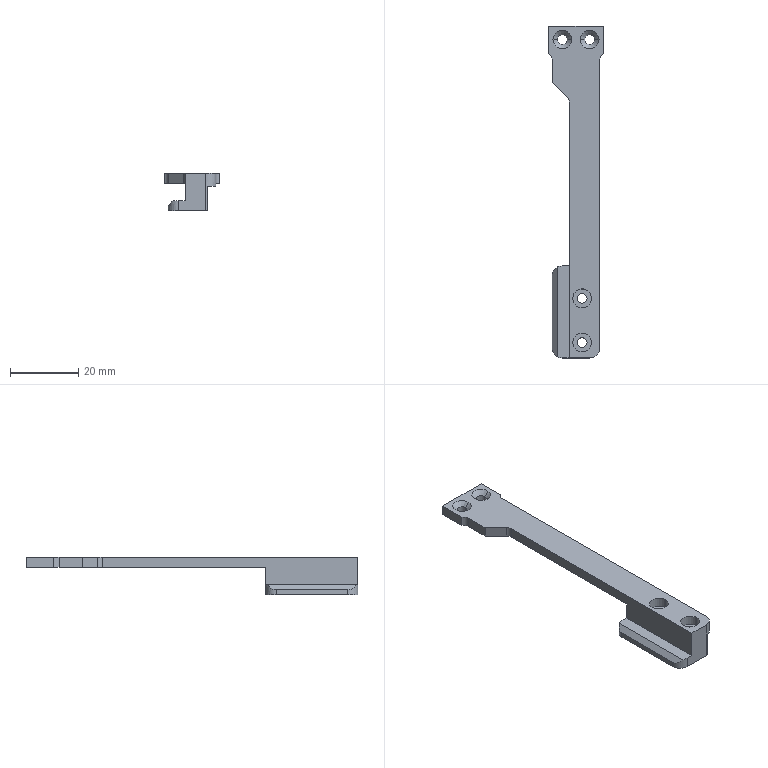Part | 1 solid | 42 faces | box 16 x 97.4 x 11 mm | volume 4478 mm3 | plane 19 | cylinder 19 | cone 4 | commonest cylinder face diameters 2.9 x8 5.5 x4 6 x4 4 x3
STEP:
#1=CARTESIAN_POINT('',(14.,3.,7.2));
#2=VERTEX_POINT('',#1);
#3=CARTESIAN_POINT('',(11.5,0.04196,7.2));
#4=VERTEX_POINT('',#3);
#5=CARTESIAN_POINT('',(11.,3.,7.2));
#6=DIRECTION('',(0.,0.,-1.));
#7=DIRECTION('',(0.,-1.,0.));
#8=AXIS2_PLACEMENT_3D('',#5,#6,#7);
#9=CIRCLE('',#8,3.);
#10=EDGE_CURVE('',#2,#4,#9,.T.);
#11=ORIENTED_EDGE('',*,*,#10,.T.);
#12=CARTESIAN_POINT('',(11.5,26.958,7.2));
#13=VERTEX_POINT('',#12);
#14=CARTESIAN_POINT('',(11.5,29.,7.2));
#15=DIRECTION('',(0.,-1.,0.));
#16=VECTOR('',#15,1000.);
#17=LINE('',#14,#16);
#18=EDGE_CURVE('',#13,#4,#17,.T.);
#19=ORIENTED_EDGE('',*,*,#18,.F.);
#20=CARTESIAN_POINT('',(14.,24.,7.2));
#21=VERTEX_POINT('',#20);
#22=CARTESIAN_POINT('',(11.,24.,7.2));
#23=DIRECTION('',(0.,0.,-1.));
#24=DIRECTION('',(0.,-1.,0.));
#25=AXIS2_PLACEMENT_3D('',#22,#23,#24);
#26=CIRCLE('',#25,3.);
#27=EDGE_CURVE('',#13,#21,#26,.T.);
#28=ORIENTED_EDGE('',*,*,#27,.T.);
#29=CARTESIAN_POINT('',(14.,29.,7.2));
#30=DIRECTION('',(0.,-1.,0.));
#31=VECTOR('',#30,1000.);
#32=LINE('',#29,#31);
#33=EDGE_CURVE('',#21,#2,#32,.T.);
#34=ORIENTED_EDGE('',*,*,#33,.T.);
#35=EDGE_LOOP('',(#11,#19,#28,#34));
#36=FACE_BOUND('',#35,.T.);
#37=CARTESIAN_POINT('',(14.,29.,7.2));
#38=DIRECTION('',(0.,0.,1.));
#39=DIRECTION('',(0.,-1.,0.));
#40=AXIS2_PLACEMENT_3D('',#37,#38,#39);
#41=PLANE('',#40);
#42=ADVANCED_FACE('',(#36),#41,.F.);
#43=CARTESIAN_POINT('',(11.5,0.04196,0.));
#44=VERTEX_POINT('',#43);
#45=CARTESIAN_POINT('',(11.5,0.04196,0.));
#46=DIRECTION('',(0.,0.,-1.));
#47=VECTOR('',#46,1000.);
#48=LINE('',#45,#47);
#49=EDGE_CURVE('',#4,#44,#48,.T.);
#50=ORIENTED_EDGE('',*,*,#49,.T.);
#51=CARTESIAN_POINT('',(11.5,26.958,0.));
#52=VERTEX_POINT('',#51);
#53=CARTESIAN_POINT('',(11.5,29.,0.));
#54=DIRECTION('',(0.,-1.,0.));
#55=VECTOR('',#54,1000.);
#56=LINE('',#53,#55);
#57=EDGE_CURVE('',#52,#44,#56,.T.);
#58=ORIENTED_EDGE('',*,*,#57,.F.);
#59=CARTESIAN_POINT('',(11.5,26.958,0.));
#60=DIRECTION('',(0.,0.,1.));
#61=VECTOR('',#60,1000.);
#62=LINE('',#59,#61);
#63=EDGE_CURVE('',#52,#13,#62,.T.);
#64=ORIENTED_EDGE('',*,*,#63,.T.);
#65=ORIENTED_EDGE('',*,*,#18,.T.);
#66=EDGE_LOOP('',(#50,#58,#64,#65));
#67=FACE_BOUND('',#66,.T.);
#68=CARTESIAN_POINT('',(11.5,29.,0.));
#69=DIRECTION('',(-1.,0.,0.));
#70=DIRECTION('',(0.,-1.,0.));
#71=AXIS2_PLACEMENT_3D('',#68,#69,#70);
#72=PLANE('',#71);
#73=ADVANCED_FACE('',(#67),#72,.F.);
#74=CARTESIAN_POINT('',(-1.,89.4,11.));
#75=VERTEX_POINT('',#74);
#76=CARTESIAN_POINT('',(0.,87.668,11.));
#77=VERTEX_POINT('',#76);
#78=CARTESIAN_POINT('',(-2.,87.668,11.));
#79=DIRECTION('',(0.,0.,-1.));
#80=DIRECTION('',(1.,0.,0.));
#81=AXIS2_PLACEMENT_3D('',#78,#79,#80);
#82=CIRCLE('',#81,2.);
#83=EDGE_CURVE('',#75,#77,#82,.T.);
#84=ORIENTED_EDGE('',*,*,#83,.F.);
#85=CARTESIAN_POINT('',(-1.,89.4,8.));
#86=VERTEX_POINT('',#85);
#87=CARTESIAN_POINT('',(-1.,89.4,-9.889));
#88=DIRECTION('',(0.,0.,1.));
#89=VECTOR('',#88,1000.);
#90=LINE('',#87,#89);
#91=EDGE_CURVE('',#86,#75,#90,.T.);
#92=ORIENTED_EDGE('',*,*,#91,.F.);
#93=CARTESIAN_POINT('',(0.,87.668,8.));
#94=VERTEX_POINT('',#93);
#95=CARTESIAN_POINT('',(-2.,87.668,8.));
#96=DIRECTION('',(0.,0.,1.));
#97=DIRECTION('',(1.,0.,0.));
#98=AXIS2_PLACEMENT_3D('',#95,#96,#97);
#99=CIRCLE('',#98,2.);
#100=EDGE_CURVE('',#94,#86,#99,.T.);
#101=ORIENTED_EDGE('',*,*,#100,.F.);
#102=CARTESIAN_POINT('',(0.,87.668,3.));
#103=DIRECTION('',(0.,0.,-1.));
#104=VECTOR('',#103,1000.);
#105=LINE('',#102,#104);
#106=EDGE_CURVE('',#77,#94,#105,.T.);
#107=ORIENTED_EDGE('',*,*,#106,.F.);
#108=EDGE_LOOP('',(#84,#92,#101,#107));
#109=FACE_BOUND('',#108,.T.);
#110=CARTESIAN_POINT('',(-2.,87.668,-9.889));
#111=DIRECTION('',(0.,0.,-1.));
#112=DIRECTION('',(-1.,0.,0.));
#113=AXIS2_PLACEMENT_3D('',#110,#111,#112);
#114=CYLINDRICAL_SURFACE('',#113,2.);
#115=ADVANCED_FACE('',(#109),#114,.F.);
#116=CARTESIAN_POINT('',(15.,89.4,8.));
#117=VERTEX_POINT('',#116);
#118=CARTESIAN_POINT('',(14.,87.668,8.));
#119=VERTEX_POINT('',#118);
#120=CARTESIAN_POINT('',(16.,87.668,8.));
#121=DIRECTION('',(0.,0.,1.));
#122=DIRECTION('',(1.,0.,0.));
#123=AXIS2_PLACEMENT_3D('',#120,#121,#122);
#124=CIRCLE('',#123,2.);
#125=EDGE_CURVE('',#117,#119,#124,.T.);
#126=ORIENTED_EDGE('',*,*,#125,.F.);
#127=CARTESIAN_POINT('',(15.,89.4,11.));
#128=VERTEX_POINT('',#127);
#129=CARTESIAN_POINT('',(15.,89.4,-9.889));
#130=DIRECTION('',(0.,0.,1.));
#131=VECTOR('',#130,1000.);
#132=LINE('',#129,#131);
#133=EDGE_CURVE('',#117,#128,#132,.T.);
#134=ORIENTED_EDGE('',*,*,#133,.T.);
#135=CARTESIAN_POINT('',(14.,87.668,11.));
#136=VERTEX_POINT('',#135);
#137=CARTESIAN_POINT('',(16.,87.668,11.));
#138=DIRECTION('',(0.,0.,-1.));
#139=DIRECTION('',(1.,0.,0.));
#140=AXIS2_PLACEMENT_3D('',#137,#138,#139);
#141=CIRCLE('',#140,2.);
#142=EDGE_CURVE('',#136,#128,#141,.T.);
#143=ORIENTED_EDGE('',*,*,#142,.F.);
#144=CARTESIAN_POINT('',(14.,87.668,0.));
#145=DIRECTION('',(0.,0.,1.));
#146=VECTOR('',#145,1000.);
#147=LINE('',#144,#146);
#148=EDGE_CURVE('',#119,#136,#147,.T.);
#149=ORIENTED_EDGE('',*,*,#148,.F.);
#150=EDGE_LOOP('',(#126,#134,#143,#149));
#151=FACE_BOUND('',#150,.T.);
#152=CARTESIAN_POINT('',(16.,87.668,-9.889));
#153=DIRECTION('',(0.,0.,1.));
#154=DIRECTION('',(1.,0.,0.));
#155=AXIS2_PLACEMENT_3D('',#152,#153,#154);
#156=CYLINDRICAL_SURFACE('',#155,2.);
#157=ADVANCED_FACE('',(#151),#156,.F.);
#158=CARTESIAN_POINT('',(1.55,93.4,9.7));
#159=VERTEX_POINT('',#158);
#160=CARTESIAN_POINT('',(0.25,93.4,11.));
#161=VERTEX_POINT('',#160);
#162=CARTESIAN_POINT('',(0.25,93.4,11.));
#163=DIRECTION('',(-0.7071,0.,0.7071));
#164=VECTOR('',#163,1000.);
#165=LINE('',#162,#164);
#166=EDGE_CURVE('',#159,#161,#165,.T.);
#167=ORIENTED_EDGE('',*,*,#166,.F.);
#168=CARTESIAN_POINT('',(4.45,93.4,9.7));
#169=VERTEX_POINT('',#168);
#170=CARTESIAN_POINT('',(3.,93.4,9.7));
#171=DIRECTION('',(0.,0.,1.));
#172=DIRECTION('',(1.,0.,0.));
#173=AXIS2_PLACEMENT_3D('',#170,#171,#172);
#174=CIRCLE('',#173,1.45);
#175=EDGE_CURVE('',#169,#159,#174,.T.);
#176=ORIENTED_EDGE('',*,*,#175,.F.);
#177=CARTESIAN_POINT('',(5.75,93.4,11.));
#178=VERTEX_POINT('',#177);
#179=CARTESIAN_POINT('',(5.75,93.4,11.));
#180=DIRECTION('',(0.7071,0.,0.7071));
#181=VECTOR('',#180,1000.);
#182=LINE('',#179,#181);
#183=EDGE_CURVE('',#169,#178,#182,.T.);
#184=ORIENTED_EDGE('',*,*,#183,.T.);
#185=CARTESIAN_POINT('',(3.,93.4,11.));
#186=DIRECTION('',(0.,0.,1.));
#187=DIRECTION('',(1.,0.,0.));
#188=AXIS2_PLACEMENT_3D('',#185,#186,#187);
#189=CIRCLE('',#188,2.75);
#190=EDGE_CURVE('',#178,#161,#189,.T.);
#191=ORIENTED_EDGE('',*,*,#190,.T.);
#192=EDGE_LOOP('',(#167,#176,#184,#191));
#193=FACE_BOUND('',#192,.T.);
#194=CARTESIAN_POINT('',(3.,93.4,11.));
#195=DIRECTION('',(0.,0.,1.));
#196=DIRECTION('',(1.,0.,0.));
#197=AXIS2_PLACEMENT_3D('',#194,#195,#196);
#198=CONICAL_SURFACE('',#197,2.75,0.7854);
#199=ADVANCED_FACE('',(#193),#198,.F.);
#200=CARTESIAN_POINT('',(1.55,93.4,8.));
#201=VERTEX_POINT('',#200);
#202=CARTESIAN_POINT('',(1.55,93.4,11.));
#203=DIRECTION('',(0.,0.,1.));
#204=VECTOR('',#203,1000.);
#205=LINE('',#202,#204);
#206=EDGE_CURVE('',#201,#159,#205,.T.);
#207=ORIENTED_EDGE('',*,*,#206,.F.);
#208=CARTESIAN_POINT('',(4.45,93.4,8.));
#209=VERTEX_POINT('',#208);
#210=CARTESIAN_POINT('',(3.,93.4,8.));
#211=DIRECTION('',(0.,0.,1.));
#212=DIRECTION('',(1.,0.,0.));
#213=AXIS2_PLACEMENT_3D('',#210,#211,#212);
#214=CIRCLE('',#213,1.45);
#215=EDGE_CURVE('',#209,#201,#214,.T.);
#216=ORIENTED_EDGE('',*,*,#215,.F.);
#217=CARTESIAN_POINT('',(4.45,93.4,11.));
#218=DIRECTION('',(0.,0.,1.));
#219=VECTOR('',#218,1000.);
#220=LINE('',#217,#219);
#221=EDGE_CURVE('',#209,#169,#220,.T.);
#222=ORIENTED_EDGE('',*,*,#221,.T.);
#223=ORIENTED_EDGE('',*,*,#175,.T.);
#224=EDGE_LOOP('',(#207,#216,#222,#223));
#225=FACE_BOUND('',#224,.T.);
#226=CARTESIAN_POINT('',(3.,93.4,11.));
#227=DIRECTION('',(0.,0.,1.));
#228=DIRECTION('',(1.,0.,0.));
#229=AXIS2_PLACEMENT_3D('',#226,#227,#228);
#230=CYLINDRICAL_SURFACE('',#229,1.45);
#231=ADVANCED_FACE('',(#225),#230,.F.);
#232=CARTESIAN_POINT('',(9.55,93.4,9.7));
#233=VERTEX_POINT('',#232);
#234=CARTESIAN_POINT('',(8.25,93.4,11.));
#235=VERTEX_POINT('',#234);
#236=CARTESIAN_POINT('',(8.25,93.4,11.));
#237=DIRECTION('',(-0.7071,0.,0.7071));
#238=VECTOR('',#237,1000.);
#239=LINE('',#236,#238);
#240=EDGE_CURVE('',#233,#235,#239,.T.);
#241=ORIENTED_EDGE('',*,*,#240,.F.);
#242=CARTESIAN_POINT('',(12.45,93.4,9.7));
#243=VERTEX_POINT('',#242);
#244=CARTESIAN_POINT('',(11.,93.4,9.7));
#245=DIRECTION('',(0.,0.,1.));
#246=DIRECTION('',(1.,0.,0.));
#247=AXIS2_PLACEMENT_3D('',#244,#245,#246);
#248=CIRCLE('',#247,1.45);
#249=EDGE_CURVE('',#243,#233,#248,.T.);
#250=ORIENTED_EDGE('',*,*,#249,.F.);
#251=CARTESIAN_POINT('',(13.75,93.4,11.));
#252=VERTEX_POINT('',#251);
#253=CARTESIAN_POINT('',(13.75,93.4,11.));
#254=DIRECTION('',(0.7071,0.,0.7071));
#255=VECTOR('',#254,1000.);
#256=LINE('',#253,#255);
#257=EDGE_CURVE('',#243,#252,#256,.T.);
#258=ORIENTED_EDGE('',*,*,#257,.T.);
#259=CARTESIAN_POINT('',(11.,93.4,11.));
#260=DIRECTION('',(0.,0.,1.));
#261=DIRECTION('',(1.,0.,0.));
#262=AXIS2_PLACEMENT_3D('',#259,#260,#261);
#263=CIRCLE('',#262,2.75);
#264=EDGE_CURVE('',#252,#235,#263,.T.);
#265=ORIENTED_EDGE('',*,*,#264,.T.);
#266=EDGE_LOOP('',(#241,#250,#258,#265));
#267=FACE_BOUND('',#266,.T.);
#268=CARTESIAN_POINT('',(11.,93.4,11.));
#269=DIRECTION('',(0.,0.,1.));
#270=DIRECTION('',(1.,0.,0.));
#271=AXIS2_PLACEMENT_3D('',#268,#269,#270);
#272=CONICAL_SURFACE('',#271,2.75,0.7854);
#273=ADVANCED_FACE('',(#267),#272,.F.);
#274=CARTESIAN_POINT('',(9.55,93.4,8.));
#275=VERTEX_POINT('',#274);
#276=CARTESIAN_POINT('',(9.55,93.4,11.));
#277=DIRECTION('',(0.,0.,1.));
#278=VECTOR('',#277,1000.);
#279=LINE('',#276,#278);
#280=EDGE_CURVE('',#275,#233,#279,.T.);
#281=ORIENTED_EDGE('',*,*,#280,.F.);
#282=CARTESIAN_POINT('',(12.45,93.4,8.));
#283=VERTEX_POINT('',#282);
#284=CARTESIAN_POINT('',(11.,93.4,8.));
#285=DIRECTION('',(0.,0.,1.));
#286=DIRECTION('',(1.,0.,0.));
#287=AXIS2_PLACEMENT_3D('',#284,#285,#286);
#288=CIRCLE('',#287,1.45);
#289=EDGE_CURVE('',#283,#275,#288,.T.);
#290=ORIENTED_EDGE('',*,*,#289,.F.);
#291=CARTESIAN_POINT('',(12.45,93.4,11.));
#292=DIRECTION('',(0.,0.,1.));
#293=VECTOR('',#292,1000.);
#294=LINE('',#291,#293);
#295=EDGE_CURVE('',#283,#243,#294,.T.);
#296=ORIENTED_EDGE('',*,*,#295,.T.);
#297=ORIENTED_EDGE('',*,*,#249,.T.);
#298=EDGE_LOOP('',(#281,#290,#296,#297));
#299=FACE_BOUND('',#298,.T.);
#300=CARTESIAN_POINT('',(11.,93.4,11.));
#301=DIRECTION('',(0.,0.,1.));
#302=DIRECTION('',(1.,0.,0.));
#303=AXIS2_PLACEMENT_3D('',#300,#301,#302);
#304=CYLINDRICAL_SURFACE('',#303,1.45);
#305=ADVANCED_FACE('',(#299),#304,.F.);
#306=CARTESIAN_POINT('',(-1.,97.4,8.));
#307=VERTEX_POINT('',#306);
#308=CARTESIAN_POINT('',(-1.,97.4,8.));
#309=DIRECTION('',(0.,1.,0.));
#310=VECTOR('',#309,1000.);
#311=LINE('',#308,#310);
#312=EDGE_CURVE('',#86,#307,#311,.T.);
#313=ORIENTED_EDGE('',*,*,#312,.F.);
#314=ORIENTED_EDGE('',*,*,#91,.T.);
#315=CARTESIAN_POINT('',(-1.,97.4,11.));
#316=VERTEX_POINT('',#315);
#317=CARTESIAN_POINT('',(-1.,97.4,11.));
#318=DIRECTION('',(0.,-1.,0.));
#319=VECTOR('',#318,1000.);
#320=LINE('',#317,#319);
#321=EDGE_CURVE('',#316,#75,#320,.T.);
#322=ORIENTED_EDGE('',*,*,#321,.F.);
#323=CARTESIAN_POINT('',(-1.,97.4,-9.889));
#324=DIRECTION('',(0.,0.,1.));
#325=VECTOR('',#324,1000.);
#326=LINE('',#323,#325);
#327=EDGE_CURVE('',#307,#316,#326,.T.);
#328=ORIENTED_EDGE('',*,*,#327,.F.);
#329=EDGE_LOOP('',(#313,#314,#322,#328));
#330=FACE_BOUND('',#329,.T.);
#331=CARTESIAN_POINT('',(-1.,97.4,-9.889));
#332=DIRECTION('',(-1.,0.,0.));
#333=DIRECTION('',(0.,-1.,0.));
#334=AXIS2_PLACEMENT_3D('',#331,#332,#333);
#335=PLANE('',#334);
#336=ADVANCED_FACE('',(#330),#335,.T.);
#337=CARTESIAN_POINT('',(15.,97.4,8.));
#338=VERTEX_POINT('',#337);
#339=CARTESIAN_POINT('',(15.,97.4,8.));
#340=DIRECTION('',(0.,-1.,0.));
#341=VECTOR('',#340,1000.);
#342=LINE('',#339,#341);
#343=EDGE_CURVE('',#338,#117,#342,.T.);
#344=ORIENTED_EDGE('',*,*,#343,.F.);
#345=CARTESIAN_POINT('',(15.,97.4,11.));
#346=VERTEX_POINT('',#345);
#347=CARTESIAN_POINT('',(15.,97.4,-9.889));
#348=DIRECTION('',(0.,0.,1.));
#349=VECTOR('',#348,1000.);
#350=LINE('',#347,#349);
#351=EDGE_CURVE('',#338,#346,#350,.T.);
#352=ORIENTED_EDGE('',*,*,#351,.T.);
#353=CARTESIAN_POINT('',(15.,97.4,11.));
#354=DIRECTION('',(0.,1.,0.));
#355=VECTOR('',#354,1000.);
#356=LINE('',#353,#355);
#357=EDGE_CURVE('',#128,#346,#356,.T.);
#358=ORIENTED_EDGE('',*,*,#357,.F.);
#359=ORIENTED_EDGE('',*,*,#133,.F.);
#360=EDGE_LOOP('',(#344,#352,#358,#359));
#361=FACE_BOUND('',#360,.T.);
#362=CARTESIAN_POINT('',(15.,97.4,-9.889));
#363=DIRECTION('',(1.,0.,0.));
#364=DIRECTION('',(0.,1.,0.));
#365=AXIS2_PLACEMENT_3D('',#362,#363,#364);
#366=PLANE('',#365);
#367=ADVANCED_FACE('',(#361),#366,.T.);
#368=CARTESIAN_POINT('',(5.,75.005,8.));
#369=VERTEX_POINT('',#368);
#370=CARTESIAN_POINT('',(4.414,76.419,8.));
#371=VERTEX_POINT('',#370);
#372=CARTESIAN_POINT('',(3.,75.005,8.));
#373=DIRECTION('',(0.,0.,1.));
#374=DIRECTION('',(1.,0.,0.));
#375=AXIS2_PLACEMENT_3D('',#372,#373,#374);
#376=CIRCLE('',#375,2.);
#377=EDGE_CURVE('',#369,#371,#376,.T.);
#378=ORIENTED_EDGE('',*,*,#377,.F.);
#379=CARTESIAN_POINT('',(5.,75.005,11.));
#380=VERTEX_POINT('',#379);
#381=CARTESIAN_POINT('',(5.,75.005,8.));
#382=DIRECTION('',(0.,0.,-1.));
#383=VECTOR('',#382,1000.);
#384=LINE('',#381,#383);
#385=EDGE_CURVE('',#380,#369,#384,.T.);
#386=ORIENTED_EDGE('',*,*,#385,.F.);
#387=CARTESIAN_POINT('',(4.414,76.419,11.));
#388=VERTEX_POINT('',#387);
#389=CARTESIAN_POINT('',(3.,75.005,11.));
#390=DIRECTION('',(0.,0.,-1.));
#391=DIRECTION('',(1.,0.,0.));
#392=AXIS2_PLACEMENT_3D('',#389,#390,#391);
#393=CIRCLE('',#392,2.);
#394=EDGE_CURVE('',#388,#380,#393,.T.);
#395=ORIENTED_EDGE('',*,*,#394,.F.);
#396=CARTESIAN_POINT('',(4.414,76.419,11.));
#397=DIRECTION('',(0.,0.,1.));
#398=VECTOR('',#397,1000.);
#399=LINE('',#396,#398);
#400=EDGE_CURVE('',#371,#388,#399,.T.);
#401=ORIENTED_EDGE('',*,*,#400,.F.);
#402=EDGE_LOOP('',(#378,#386,#395,#401));
#403=FACE_BOUND('',#402,.T.);
#404=CARTESIAN_POINT('',(3.,75.005,3.));
#405=DIRECTION('',(0.,0.,-1.));
#406=DIRECTION('',(-1.,0.,0.));
#407=AXIS2_PLACEMENT_3D('',#404,#405,#406);
#408=CYLINDRICAL_SURFACE('',#407,2.);
#409=ADVANCED_FACE('',(#403),#408,.F.);
#410=CARTESIAN_POINT('',(6.049,4.5,8.1));
#411=VERTEX_POINT('',#410);
#412=CARTESIAN_POINT('',(6.049,4.5,11.));
#413=VERTEX_POINT('',#412);
#414=CARTESIAN_POINT('',(6.049,4.5,11.));
#415=DIRECTION('',(0.,0.,1.));
#416=VECTOR('',#415,1000.);
#417=LINE('',#414,#416);
#418=EDGE_CURVE('',#411,#413,#417,.T.);
#419=ORIENTED_EDGE('',*,*,#418,.F.);
#420=CARTESIAN_POINT('',(11.549,4.5,8.1));
#421=VERTEX_POINT('',#420);
#422=CARTESIAN_POINT('',(8.799,4.5,8.1));
#423=DIRECTION('',(0.,0.,1.));
#424=DIRECTION('',(1.,0.,0.));
#425=AXIS2_PLACEMENT_3D('',#422,#423,#424);
#426=CIRCLE('',#425,2.75);
#427=EDGE_CURVE('',#421,#411,#426,.T.);
#428=ORIENTED_EDGE('',*,*,#427,.F.);
#429=CARTESIAN_POINT('',(11.549,4.5,11.));
#430=VERTEX_POINT('',#429);
#431=CARTESIAN_POINT('',(11.549,4.5,11.));
#432=DIRECTION('',(0.,0.,1.));
#433=VECTOR('',#432,1000.);
#434=LINE('',#431,#433);
#435=EDGE_CURVE('',#421,#430,#434,.T.);
#436=ORIENTED_EDGE('',*,*,#435,.T.);
#437=CARTESIAN_POINT('',(8.799,4.5,11.));
#438=DIRECTION('',(0.,0.,1.));
#439=DIRECTION('',(1.,0.,0.));
#440=AXIS2_PLACEMENT_3D('',#437,#438,#439);
#441=CIRCLE('',#440,2.75);
#442=EDGE_CURVE('',#430,#413,#441,.T.);
#443=ORIENTED_EDGE('',*,*,#442,.T.);
#444=EDGE_LOOP('',(#419,#428,#436,#443));
#445=FACE_BOUND('',#444,.T.);
#446=CARTESIAN_POINT('',(8.799,4.5,11.));
#447=DIRECTION('',(0.,0.,1.));
#448=DIRECTION('',(1.,0.,0.));
#449=AXIS2_PLACEMENT_3D('',#446,#447,#448);
#450=CYLINDRICAL_SURFACE('',#449,2.75);
#451=ADVANCED_FACE('',(#445),#450,.F.);
#452=ORIENTED_EDGE('',*,*,#427,.T.);
#453=CARTESIAN_POINT('',(8.799,4.5,8.1));
#454=DIRECTION('',(0.,0.,1.));
#455=DIRECTION('',(1.,0.,0.));
#456=AXIS2_PLACEMENT_3D('',#453,#454,#455);
#457=CIRCLE('',#456,2.75);
#458=EDGE_CURVE('',#411,#421,#457,.T.);
#459=ORIENTED_EDGE('',*,*,#458,.T.);
#460=EDGE_LOOP('',(#452,#459));
#461=FACE_BOUND('',#460,.T.);
#462=CARTESIAN_POINT('',(10.249,4.5,8.1));
#463=VERTEX_POINT('',#462);
#464=CARTESIAN_POINT('',(7.349,4.5,8.1));
#465=VERTEX_POINT('',#464);
#466=CARTESIAN_POINT('',(8.799,4.5,8.1));
#467=DIRECTION('',(0.,0.,1.));
#468=DIRECTION('',(1.,0.,0.));
#469=AXIS2_PLACEMENT_3D('',#466,#467,#468);
#470=CIRCLE('',#469,1.45);
#471=EDGE_CURVE('',#463,#465,#470,.T.);
#472=ORIENTED_EDGE('',*,*,#471,.F.);
#473=CARTESIAN_POINT('',(8.799,4.5,8.1));
#474=DIRECTION('',(0.,0.,1.));
#475=DIRECTION('',(1.,0.,0.));
#476=AXIS2_PLACEMENT_3D('',#473,#474,#475);
#477=CIRCLE('',#476,1.45);
#478=EDGE_CURVE('',#465,#463,#477,.T.);
#479=ORIENTED_EDGE('',*,*,#478,.F.);
#480=EDGE_LOOP('',(#472,#479));
#481=FACE_BOUND('',#480,.T.);
#482=CARTESIAN_POINT('',(10.249,4.5,8.1));
#483=DIRECTION('',(0.,0.,-1.));
#484=DIRECTION('',(-1.,0.,0.));
#485=AXIS2_PLACEMENT_3D('',#482,#483,#484);
#486=PLANE('',#485);
#487=ADVANCED_FACE('',(#461,#481),#486,.F.);
#488=CARTESIAN_POINT('',(7.349,4.5,0.));
#489=VERTEX_POINT('',#488);
#490=CARTESIAN_POINT('',(7.349,4.5,11.));
#491=DIRECTION('',(0.,0.,1.));
#492=VECTOR('',#491,1000.);
#493=LINE('',#490,#492);
#494=EDGE_CURVE('',#489,#465,#493,.T.);
#495=ORIENTED_EDGE('',*,*,#494,.F.);
#496=CARTESIAN_POINT('',(10.249,4.5,0.));
#497=VERTEX_POINT('',#496);
#498=CARTESIAN_POINT('',(8.799,4.5,0.));
#499=DIRECTION('',(0.,0.,-1.));
#500=DIRECTION('',(-1.,0.,0.));
#501=AXIS2_PLACEMENT_3D('',#498,#499,#500);
#502=CIRCLE('',#501,1.45);
#503=EDGE_CURVE('',#489,#497,#502,.T.);
#504=ORIENTED_EDGE('',*,*,#503,.T.);
#505=CARTESIAN_POINT('',(10.249,4.5,11.));
#506=DIRECTION('',(0.,0.,1.));
#507=VECTOR('',#506,1000.);
#508=LINE('',#505,#507);
#509=EDGE_CURVE('',#497,#463,#508,.T.);
#510=ORIENTED_EDGE('',*,*,#509,.T.);
#511=ORIENTED_EDGE('',*,*,#471,.T.);
#512=EDGE_LOOP('',(#495,#504,#510,#511));
#513=FACE_BOUND('',#512,.T.);
#514=CARTESIAN_POINT('',(8.799,4.5,11.));
#515=DIRECTION('',(0.,0.,1.));
#516=DIRECTION('',(1.,0.,0.));
#517=AXIS2_PLACEMENT_3D('',#514,#515,#516);
#518=CYLINDRICAL_SURFACE('',#517,1.45);
#519=ADVANCED_FACE('',(#513),#518,.F.);
#520=CARTESIAN_POINT('',(6.049,17.5,8.1));
#521=VERTEX_POINT('',#520);
#522=CARTESIAN_POINT('',(6.049,17.5,11.));
#523=VERTEX_POINT('',#522);
#524=CARTESIAN_POINT('',(6.049,17.5,11.));
#525=DIRECTION('',(0.,0.,1.));
#526=VECTOR('',#525,1000.);
#527=LINE('',#524,#526);
#528=EDGE_CURVE('',#521,#523,#527,.T.);
#529=ORIENTED_EDGE('',*,*,#528,.F.);
#530=CARTESIAN_POINT('',(11.549,17.5,8.1));
#531=VERTEX_POINT('',#530);
#532=CARTESIAN_POINT('',(8.799,17.5,8.1));
#533=DIRECTION('',(0.,0.,1.));
#534=DIRECTION('',(1.,0.,0.));
#535=AXIS2_PLACEMENT_3D('',#532,#533,#534);
#536=CIRCLE('',#535,2.75);
#537=EDGE_CURVE('',#531,#521,#536,.T.);
#538=ORIENTED_EDGE('',*,*,#537,.F.);
#539=CARTESIAN_POINT('',(11.549,17.5,11.));
#540=VERTEX_POINT('',#539);
#541=CARTESIAN_POINT('',(11.549,17.5,11.));
#542=DIRECTION('',(0.,0.,1.));
#543=VECTOR('',#542,1000.);
#544=LINE('',#541,#543);
#545=EDGE_CURVE('',#531,#540,#544,.T.);
#546=ORIENTED_EDGE('',*,*,#545,.T.);
#547=CARTESIAN_POINT('',(8.799,17.5,11.));
#548=DIRECTION('',(0.,0.,1.));
#549=DIRECTION('',(1.,0.,0.));
#550=AXIS2_PLACEMENT_3D('',#547,#548,#549);
#551=CIRCLE('',#550,2.75);
#552=EDGE_CURVE('',#540,#523,#551,.T.);
#553=ORIENTED_EDGE('',*,*,#552,.T.);
#554=EDGE_LOOP('',(#529,#538,#546,#553));
#555=FACE_BOUND('',#554,.T.);
#556=CARTESIAN_POINT('',(8.799,17.5,11.));
#557=DIRECTION('',(0.,0.,1.));
#558=DIRECTION('',(1.,0.,0.));
#559=AXIS2_PLACEMENT_3D('',#556,#557,#558);
#560=CYLINDRICAL_SURFACE('',#559,2.75);
#561=ADVANCED_FACE('',(#555),#560,.F.);
#562=ORIENTED_EDGE('',*,*,#537,.T.);
#563=CARTESIAN_POINT('',(8.799,17.5,8.1));
#564=DIRECTION('',(0.,0.,1.));
#565=DIRECTION('',(1.,0.,0.));
#566=AXIS2_PLACEMENT_3D('',#563,#564,#565);
#567=CIRCLE('',#566,2.75);
#568=EDGE_CURVE('',#521,#531,#567,.T.);
#569=ORIENTED_EDGE('',*,*,#568,.T.);
#570=EDGE_LOOP('',(#562,#569));
#571=FACE_BOUND('',#570,.T.);
#572=CARTESIAN_POINT('',(10.249,17.5,8.1));
#573=VERTEX_POINT('',#572);
#574=CARTESIAN_POINT('',(7.349,17.5,8.1));
#575=VERTEX_POINT('',#574);
#576=CARTESIAN_POINT('',(8.799,17.5,8.1));
#577=DIRECTION('',(0.,0.,1.));
#578=DIRECTION('',(1.,0.,0.));
#579=AXIS2_PLACEMENT_3D('',#576,#577,#578);
#580=CIRCLE('',#579,1.45);
#581=EDGE_CURVE('',#573,#575,#580,.T.);
#582=ORIENTED_EDGE('',*,*,#581,.F.);
#583=CARTESIAN_POINT('',(8.799,17.5,8.1));
#584=DIRECTION('',(0.,0.,1.));
#585=DIRECTION('',(1.,0.,0.));
#586=AXIS2_PLACEMENT_3D('',#583,#584,#585);
#587=CIRCLE('',#586,1.45);
#588=EDGE_CURVE('',#575,#573,#587,.T.);
#589=ORIENTED_EDGE('',*,*,#588,.F.);
#590=EDGE_LOOP('',(#582,#589));
#591=FACE_BOUND('',#590,.T.);
#592=CARTESIAN_POINT('',(10.249,17.5,8.1));
#593=DIRECTION('',(0.,0.,-1.));
#594=DIRECTION('',(-1.,0.,0.));
#595=AXIS2_PLACEMENT_3D('',#592,#593,#594);
#596=PLANE('',#595);
#597=ADVANCED_FACE('',(#571,#591),#596,.F.);
#598=CARTESIAN_POINT('',(7.349,17.5,0.));
#599=VERTEX_POINT('',#598);
#600=CARTESIAN_POINT('',(7.349,17.5,11.));
#601=DIRECTION('',(0.,0.,1.));
#602=VECTOR('',#601,1000.);
#603=LINE('',#600,#602);
#604=EDGE_CURVE('',#599,#575,#603,.T.);
#605=ORIENTED_EDGE('',*,*,#604,.F.);
#606=CARTESIAN_POINT('',(10.249,17.5,0.));
#607=VERTEX_POINT('',#606);
#608=CARTESIAN_POINT('',(8.799,17.5,0.));
#609=DIRECTION('',(0.,0.,-1.));
#610=DIRECTION('',(-1.,0.,0.));
#611=AXIS2_PLACEMENT_3D('',#608,#609,#610);
#612=CIRCLE('',#611,1.45);
#613=EDGE_CURVE('',#599,#607,#612,.T.);
#614=ORIENTED_EDGE('',*,*,#613,.T.);
#615=CARTESIAN_POINT('',(10.249,17.5,11.));
#616=DIRECTION('',(0.,0.,1.));
#617=VECTOR('',#616,1000.);
#618=LINE('',#615,#617);
#619=EDGE_CURVE('',#607,#573,#618,.T.);
#620=ORIENTED_EDGE('',*,*,#619,.T.);
#621=ORIENTED_EDGE('',*,*,#581,.T.);
#622=EDGE_LOOP('',(#605,#614,#620,#621));
#623=FACE_BOUND('',#622,.T.);
#624=CARTESIAN_POINT('',(8.799,17.5,11.));
#625=DIRECTION('',(0.,0.,1.));
#626=DIRECTION('',(1.,0.,0.));
#627=AXIS2_PLACEMENT_3D('',#624,#625,#626);
#628=CYLINDRICAL_SURFACE('',#627,1.45);
#629=ADVANCED_FACE('',(#623),#628,.F.);
#630=ORIENTED_EDGE('',*,*,#63,.F.);
#631=CARTESIAN_POINT('',(11.,27.,0.));
#632=VERTEX_POINT('',#631);
#633=CARTESIAN_POINT('',(11.,24.,0.));
#634=DIRECTION('',(0.,0.,-1.));
#635=DIRECTION('',(-1.,0.,0.));
#636=AXIS2_PLACEMENT_3D('',#633,#634,#635);
#637=CIRCLE('',#636,3.);
#638=EDGE_CURVE('',#632,#52,#637,.T.);
#639=ORIENTED_EDGE('',*,*,#638,.F.);
#640=CARTESIAN_POINT('',(11.,27.,8.));
#641=VERTEX_POINT('',#640);
#642=CARTESIAN_POINT('',(11.,27.,11.));
#643=DIRECTION('',(0.,0.,-1.));
#644=VECTOR('',#643,1000.);
#645=LINE('',#642,#644);
#646=EDGE_CURVE('',#641,#632,#645,.T.);
#647=ORIENTED_EDGE('',*,*,#646,.F.);
#648=CARTESIAN_POINT('',(14.,24.,8.));
#649=VERTEX_POINT('',#648);
#650=CARTESIAN_POINT('',(11.,24.,8.));
#651=DIRECTION('',(0.,0.,1.));
#652=DIRECTION('',(1.,0.,0.));
#653=AXIS2_PLACEMENT_3D('',#650,#651,#652);
#654=CIRCLE('',#653,3.);
#655=EDGE_CURVE('',#649,#641,#654,.T.);
#656=ORIENTED_EDGE('',*,*,#655,.F.);
#657=CARTESIAN_POINT('',(14.,24.,0.));
#658=DIRECTION('',(0.,0.,1.));
#659=VECTOR('',#658,1000.);
#660=LINE('',#657,#659);
#661=EDGE_CURVE('',#21,#649,#660,.T.);
#662=ORIENTED_EDGE('',*,*,#661,.F.);
#663=ORIENTED_EDGE('',*,*,#27,.F.);
#664=EDGE_LOOP('',(#630,#639,#647,#656,#662,#663));
#665=FACE_BOUND('',#664,.T.);
#666=CARTESIAN_POINT('',(11.,24.,0.));
#667=DIRECTION('',(0.,0.,1.));
#668=DIRECTION('',(1.,0.,0.));
#669=AXIS2_PLACEMENT_3D('',#666,#667,#668);
#670=CYLINDRICAL_SURFACE('',#669,3.);
#671=ADVANCED_FACE('',(#665),#670,.T.);
#672=ORIENTED_EDGE('',*,*,#49,.F.);
#673=ORIENTED_EDGE('',*,*,#10,.F.);
#674=CARTESIAN_POINT('',(14.,3.,11.));
#675=VERTEX_POINT('',#674);
#676=CARTESIAN_POINT('',(14.,3.,0.));
#677=DIRECTION('',(0.,0.,-1.));
#678=VECTOR('',#677,1000.);
#679=LINE('',#676,#678);
#680=EDGE_CURVE('',#675,#2,#679,.T.);
#681=ORIENTED_EDGE('',*,*,#680,.F.);
#682=CARTESIAN_POINT('',(11.,0.,11.));
#683=VERTEX_POINT('',#682);
#684=CARTESIAN_POINT('',(11.,3.,11.));
#685=DIRECTION('',(0.,0.,1.));
#686=DIRECTION('',(1.,0.,0.));
#687=AXIS2_PLACEMENT_3D('',#684,#685,#686);
#688=CIRCLE('',#687,3.);
#689=EDGE_CURVE('',#683,#675,#688,.T.);
#690=ORIENTED_EDGE('',*,*,#689,.F.);
#691=CARTESIAN_POINT('',(11.,0.,0.));
#692=VERTEX_POINT('',#691);
#693=CARTESIAN_POINT('',(11.,0.,3.));
#694=DIRECTION('',(0.,0.,1.));
#695=VECTOR('',#694,1000.);
#696=LINE('',#693,#695);
#697=EDGE_CURVE('',#692,#683,#696,.T.);
#698=ORIENTED_EDGE('',*,*,#697,.F.);
#699=CARTESIAN_POINT('',(11.,3.,0.));
#700=DIRECTION('',(0.,0.,-1.));
#701=DIRECTION('',(-1.,0.,0.));
#702=AXIS2_PLACEMENT_3D('',#699,#700,#701);
#703=CIRCLE('',#702,3.);
#704=EDGE_CURVE('',#44,#692,#703,.T.);
#705=ORIENTED_EDGE('',*,*,#704,.F.);
#706=EDGE_LOOP('',(#672,#673,#681,#690,#698,#705));
#707=FACE_BOUND('',#706,.T.);
#708=CARTESIAN_POINT('',(11.,3.,0.));
#709=DIRECTION('',(0.,0.,-1.));
#710=DIRECTION('',(-1.,0.,0.));
#711=AXIS2_PLACEMENT_3D('',#708,#709,#710);
#712=CYLINDRICAL_SURFACE('',#711,3.);
#713=ADVANCED_FACE('',(#707),#712,.T.);
#714=CARTESIAN_POINT('',(3.,27.,3.));
#715=VERTEX_POINT('',#714);
#716=CARTESIAN_POINT('',(1.5,26.598,3.));
#717=VERTEX_POINT('',#716);
#718=CARTESIAN_POINT('',(3.,24.,3.));
#719=DIRECTION('',(0.,0.,1.));
#720=DIRECTION('',(-1.,0.,0.));
#721=AXIS2_PLACEMENT_3D('',#718,#719,#720);
#722=CIRCLE('',#721,3.);
#723=EDGE_CURVE('',#715,#717,#722,.T.);
#724=ORIENTED_EDGE('',*,*,#723,.F.);
#725=CARTESIAN_POINT('',(3.,27.,0.));
#726=VERTEX_POINT('',#725);
#727=CARTESIAN_POINT('',(3.,27.,11.));
#728=DIRECTION('',(0.,0.,1.));
#729=VECTOR('',#728,1000.);
#730=LINE('',#727,#729);
#731=EDGE_CURVE('',#726,#715,#730,.T.);
#732=ORIENTED_EDGE('',*,*,#731,.F.);
#733=CARTESIAN_POINT('',(0.,24.,0.));
#734=VERTEX_POINT('',#733);
#735=CARTESIAN_POINT('',(3.,24.,0.));
#736=DIRECTION('',(0.,0.,-1.));
#737=DIRECTION('',(-1.,0.,0.));
#738=AXIS2_PLACEMENT_3D('',#735,#736,#737);
#739=CIRCLE('',#738,3.);
#740=EDGE_CURVE('',#734,#726,#739,.T.);
#741=ORIENTED_EDGE('',*,*,#740,.F.);
#742=CARTESIAN_POINT('',(0.,24.,1.5));
#743=VERTEX_POINT('',#742);
#744=CARTESIAN_POINT('',(0.,24.,3.));
#745=DIRECTION('',(0.,0.,-1.));
#746=VECTOR('',#745,1000.);
#747=LINE('',#744,#746);
#748=EDGE_CURVE('',#743,#734,#747,.T.);
#749=ORIENTED_EDGE('',*,*,#748,.F.);
#750=CARTESIAN_POINT('',(1.5,26.598,3.));
#751=CARTESIAN_POINT('',(0.549,26.049,2.049));
#752=CARTESIAN_POINT('',(0.,25.098,1.5));
#753=CARTESIAN_POINT('',(0.,24.,1.5));
#754=(BOUNDED_CURVE()B_SPLINE_CURVE(3,(#750,#751,#752,#753),.UNSPECIFIED.,.F.,.F.)B_SPLINE_CURVE_WITH_KNOTS((4,4),(5.236,6.283),.UNSPECIFIED.)CURVE()GEOMETRIC_REPRESENTATION_ITEM()RATIONAL_B_SPLINE_CURVE((1.,0.9107,0.9107,1.))REPRESENTATION_ITEM(''));
#755=EDGE_CURVE('',#717,#743,#754,.T.);
#756=ORIENTED_EDGE('',*,*,#755,.F.);
#757=EDGE_LOOP('',(#724,#732,#741,#749,#756));
#758=FACE_BOUND('',#757,.T.);
#759=CARTESIAN_POINT('',(3.,24.,3.));
#760=DIRECTION('',(0.,0.,-1.));
#761=DIRECTION('',(-1.,0.,0.));
#762=AXIS2_PLACEMENT_3D('',#759,#760,#761);
#763=CYLINDRICAL_SURFACE('',#762,3.);
#764=ADVANCED_FACE('',(#758),#763,.T.);
#765=CARTESIAN_POINT('',(0.,3.,1.5));
#766=VERTEX_POINT('',#765);
#767=CARTESIAN_POINT('',(1.5,0.4019,3.));
#768=VERTEX_POINT('',#767);
#769=CARTESIAN_POINT('',(0.,3.,1.5));
#770=CARTESIAN_POINT('',(0.,1.902,1.5));
#771=CARTESIAN_POINT('',(0.549,0.951,2.049));
#772=CARTESIAN_POINT('',(1.5,0.4019,3.));
#773=(BOUNDED_CURVE()B_SPLINE_CURVE(3,(#769,#770,#771,#772),.UNSPECIFIED.,.F.,.F.)B_SPLINE_CURVE_WITH_KNOTS((4,4),(0.,1.047),.UNSPECIFIED.)CURVE()GEOMETRIC_REPRESENTATION_ITEM()RATIONAL_B_SPLINE_CURVE((1.,0.9107,0.9107,1.))REPRESENTATION_ITEM(''));
#774=EDGE_CURVE('',#766,#768,#773,.T.);
#775=ORIENTED_EDGE('',*,*,#774,.F.);
#776=CARTESIAN_POINT('',(0.,3.,0.));
#777=VERTEX_POINT('',#776);
#778=CARTESIAN_POINT('',(0.,3.,3.));
#779=DIRECTION('',(0.,0.,1.));
#780=VECTOR('',#779,1000.);
#781=LINE('',#778,#780);
#782=EDGE_CURVE('',#777,#766,#781,.T.);
#783=ORIENTED_EDGE('',*,*,#782,.F.);
#784=CARTESIAN_POINT('',(3.,0.,0.));
#785=VERTEX_POINT('',#784);
#786=CARTESIAN_POINT('',(3.,3.,0.));
#787=DIRECTION('',(0.,0.,-1.));
#788=DIRECTION('',(-1.,0.,0.));
#789=AXIS2_PLACEMENT_3D('',#786,#787,#788);
#790=CIRCLE('',#789,3.);
#791=EDGE_CURVE('',#785,#777,#790,.T.);
#792=ORIENTED_EDGE('',*,*,#791,.F.);
#793=CARTESIAN_POINT('',(3.,0.,3.));
#794=VERTEX_POINT('',#793);
#795=CARTESIAN_POINT('',(3.,0.,3.));
#796=DIRECTION('',(0.,0.,-1.));
#797=VECTOR('',#796,1000.);
#798=LINE('',#795,#797);
#799=EDGE_CURVE('',#794,#785,#798,.T.);
#800=ORIENTED_EDGE('',*,*,#799,.F.);
#801=CARTESIAN_POINT('',(3.,3.,3.));
#802=DIRECTION('',(0.,0.,1.));
#803=DIRECTION('',(-1.,0.,0.));
#804=AXIS2_PLACEMENT_3D('',#801,#802,#803);
#805=CIRCLE('',#804,3.);
#806=EDGE_CURVE('',#768,#794,#805,.T.);
#807=ORIENTED_EDGE('',*,*,#806,.F.);
#808=EDGE_LOOP('',(#775,#783,#792,#800,#807));
#809=FACE_BOUND('',#808,.T.);
#810=CARTESIAN_POINT('',(3.,3.,3.));
#811=DIRECTION('',(0.,0.,-1.));
#812=DIRECTION('',(-1.,0.,0.));
#813=AXIS2_PLACEMENT_3D('',#810,#811,#812);
#814=CYLINDRICAL_SURFACE('',#813,3.);
#815=ADVANCED_FACE('',(#809),#814,.T.);
#816=CARTESIAN_POINT('',(0.,0.,1.5));
#817=DIRECTION('',(0.,1.,0.));
#818=VECTOR('',#817,1000.);
#819=LINE('',#816,#818);
#820=EDGE_CURVE('',#766,#743,#819,.T.);
#821=ORIENTED_EDGE('',*,*,#820,.F.);
#822=ORIENTED_EDGE('',*,*,#774,.T.);
#823=CARTESIAN_POINT('',(1.5,0.,3.));
#824=DIRECTION('',(0.,-1.,0.));
#825=VECTOR('',#824,1000.);
#826=LINE('',#823,#825);
#827=EDGE_CURVE('',#717,#768,#826,.T.);
#828=ORIENTED_EDGE('',*,*,#827,.F.);
#829=ORIENTED_EDGE('',*,*,#755,.T.);
#830=EDGE_LOOP('',(#821,#822,#828,#829));
#831=FACE_BOUND('',#830,.T.);
#832=CARTESIAN_POINT('',(1.5,0.,3.));
#833=DIRECTION('',(0.7071,0.,-0.7071));
#834=DIRECTION('',(0.,-1.,0.));
#835=AXIS2_PLACEMENT_3D('',#832,#833,#834);
#836=PLANE('',#835);
#837=ADVANCED_FACE('',(#831),#836,.F.);
#838=CARTESIAN_POINT('',(5.,0.,11.));
#839=VERTEX_POINT('',#838);
#840=CARTESIAN_POINT('',(5.,0.,11.));
#841=DIRECTION('',(0.,1.,0.));
#842=VECTOR('',#841,1000.);
#843=LINE('',#840,#842);
#844=EDGE_CURVE('',#839,#380,#843,.T.);
#845=ORIENTED_EDGE('',*,*,#844,.T.);
#846=ORIENTED_EDGE('',*,*,#385,.T.);
#847=CARTESIAN_POINT('',(5.,27.,8.));
#848=VERTEX_POINT('',#847);
#849=CARTESIAN_POINT('',(5.,0.,8.));
#850=DIRECTION('',(0.,1.,0.));
#851=VECTOR('',#850,1000.);
#852=LINE('',#849,#851);
#853=EDGE_CURVE('',#848,#369,#852,.T.);
#854=ORIENTED_EDGE('',*,*,#853,.F.);
#855=CARTESIAN_POINT('',(5.,27.,3.));
#856=VERTEX_POINT('',#855);
#857=CARTESIAN_POINT('',(5.,27.,11.));
#858=DIRECTION('',(0.,0.,1.));
#859=VECTOR('',#858,1000.);
#860=LINE('',#857,#859);
#861=EDGE_CURVE('',#856,#848,#860,.T.);
#862=ORIENTED_EDGE('',*,*,#861,.F.);
#863=CARTESIAN_POINT('',(5.,0.,3.));
#864=VERTEX_POINT('',#863);
#865=CARTESIAN_POINT('',(5.,0.,3.));
#866=DIRECTION('',(0.,1.,0.));
#867=VECTOR('',#866,1000.);
#868=LINE('',#865,#867);
#869=EDGE_CURVE('',#864,#856,#868,.T.);
#870=ORIENTED_EDGE('',*,*,#869,.F.);
#871=CARTESIAN_POINT('',(5.,0.,3.));
#872=DIRECTION('',(0.,0.,1.));
#873=VECTOR('',#872,1000.);
#874=LINE('',#871,#873);
#875=EDGE_CURVE('',#864,#839,#874,.T.);
#876=ORIENTED_EDGE('',*,*,#875,.T.);
#877=EDGE_LOOP('',(#845,#846,#854,#862,#870,#876));
#878=FACE_BOUND('',#877,.T.);
#879=CARTESIAN_POINT('',(5.,0.,3.));
#880=DIRECTION('',(1.,0.,0.));
#881=DIRECTION('',(0.,0.,-1.));
#882=AXIS2_PLACEMENT_3D('',#879,#880,#881);
#883=PLANE('',#882);
#884=ADVANCED_FACE('',(#878),#883,.F.);
#885=CARTESIAN_POINT('',(0.,80.833,8.));
#886=VERTEX_POINT('',#885);
#887=CARTESIAN_POINT('',(40.417,40.417,8.));
#888=DIRECTION('',(-0.7071,0.7071,0.));
#889=VECTOR('',#888,1000.);
#890=LINE('',#887,#889);
#891=EDGE_CURVE('',#371,#886,#890,.T.);
#892=ORIENTED_EDGE('',*,*,#891,.F.);
#893=ORIENTED_EDGE('',*,*,#400,.T.);
#894=CARTESIAN_POINT('',(0.,80.833,11.));
#895=VERTEX_POINT('',#894);
#896=CARTESIAN_POINT('',(0.,80.833,11.));
#897=DIRECTION('',(-0.7071,0.7071,0.));
#898=VECTOR('',#897,1000.);
#899=LINE('',#896,#898);
#900=EDGE_CURVE('',#388,#895,#899,.T.);
#901=ORIENTED_EDGE('',*,*,#900,.T.);
#902=CARTESIAN_POINT('',(0.,80.833,3.));
#903=DIRECTION('',(0.,0.,1.));
#904=VECTOR('',#903,1000.);
#905=LINE('',#902,#904);
#906=EDGE_CURVE('',#886,#895,#905,.T.);
#907=ORIENTED_EDGE('',*,*,#906,.F.);
#908=EDGE_LOOP('',(#892,#893,#901,#907));
#909=FACE_BOUND('',#908,.T.);
#910=CARTESIAN_POINT('',(0.,80.833,3.));
#911=DIRECTION('',(0.7071,0.7071,0.));
#912=DIRECTION('',(-0.7071,0.7071,0.));
#913=AXIS2_PLACEMENT_3D('',#910,#911,#912);
#914=PLANE('',#913);
#915=ADVANCED_FACE('',(#909),#914,.F.);
#916=ORIENTED_EDGE('',*,*,#827,.T.);
#917=ORIENTED_EDGE('',*,*,#806,.T.);
#918=CARTESIAN_POINT('',(0.,0.,3.));
#919=DIRECTION('',(1.,0.,0.));
#920=VECTOR('',#919,1000.);
#921=LINE('',#918,#920);
#922=EDGE_CURVE('',#794,#864,#921,.T.);
#923=ORIENTED_EDGE('',*,*,#922,.T.);
#924=ORIENTED_EDGE('',*,*,#869,.T.);
#925=CARTESIAN_POINT('',(14.,27.,3.));
#926=DIRECTION('',(1.,0.,0.));
#927=VECTOR('',#926,1000.);
#928=LINE('',#925,#927);
#929=EDGE_CURVE('',#715,#856,#928,.T.);
#930=ORIENTED_EDGE('',*,*,#929,.F.);
#931=ORIENTED_EDGE('',*,*,#723,.T.);
#932=EDGE_LOOP('',(#916,#917,#923,#924,#930,#931));
#933=FACE_BOUND('',#932,.T.);
#934=CARTESIAN_POINT('',(0.,0.,3.));
#935=DIRECTION('',(0.,0.,-1.));
#936=DIRECTION('',(-1.,0.,0.));
#937=AXIS2_PLACEMENT_3D('',#934,#935,#936);
#938=PLANE('',#937);
#939=ADVANCED_FACE('',(#933),#938,.F.);
#940=CARTESIAN_POINT('',(0.,0.,8.));
#941=DIRECTION('',(0.,-1.,0.));
#942=VECTOR('',#941,1000.);
#943=LINE('',#940,#942);
#944=EDGE_CURVE('',#94,#886,#943,.T.);
#945=ORIENTED_EDGE('',*,*,#944,.F.);
#946=ORIENTED_EDGE('',*,*,#100,.T.);
#947=ORIENTED_EDGE('',*,*,#312,.T.);
#948=CARTESIAN_POINT('',(14.,97.4,8.));
#949=DIRECTION('',(-1.,0.,0.));
#950=VECTOR('',#949,1000.);
#951=LINE('',#948,#950);
#952=EDGE_CURVE('',#338,#307,#951,.T.);
#953=ORIENTED_EDGE('',*,*,#952,.F.);
#954=ORIENTED_EDGE('',*,*,#343,.T.);
#955=ORIENTED_EDGE('',*,*,#125,.T.);
#956=CARTESIAN_POINT('',(14.,27.,8.));
#957=DIRECTION('',(0.,1.,0.));
#958=VECTOR('',#957,1000.);
#959=LINE('',#956,#958);
#960=EDGE_CURVE('',#649,#119,#959,.T.);
#961=ORIENTED_EDGE('',*,*,#960,.F.);
#962=ORIENTED_EDGE('',*,*,#655,.T.);
#963=CARTESIAN_POINT('',(14.,27.,8.));
#964=DIRECTION('',(1.,0.,0.));
#965=VECTOR('',#964,1000.);
#966=LINE('',#963,#965);
#967=EDGE_CURVE('',#848,#641,#966,.T.);
#968=ORIENTED_EDGE('',*,*,#967,.F.);
#969=ORIENTED_EDGE('',*,*,#853,.T.);
#970=ORIENTED_EDGE('',*,*,#377,.T.);
#971=ORIENTED_EDGE('',*,*,#891,.T.);
#972=EDGE_LOOP('',(#945,#946,#947,#953,#954,#955,#961,#962,#968,#969,#970,#971));
#973=FACE_BOUND('',#972,.T.);
#974=ORIENTED_EDGE('',*,*,#289,.T.);
#975=CARTESIAN_POINT('',(11.,93.4,8.));
#976=DIRECTION('',(0.,0.,1.));
#977=DIRECTION('',(1.,0.,0.));
#978=AXIS2_PLACEMENT_3D('',#975,#976,#977);
#979=CIRCLE('',#978,1.45);
#980=EDGE_CURVE('',#275,#283,#979,.T.);
#981=ORIENTED_EDGE('',*,*,#980,.T.);
#982=EDGE_LOOP('',(#974,#981));
#983=FACE_BOUND('',#982,.T.);
#984=ORIENTED_EDGE('',*,*,#215,.T.);
#985=CARTESIAN_POINT('',(3.,93.4,8.));
#986=DIRECTION('',(0.,0.,1.));
#987=DIRECTION('',(1.,0.,0.));
#988=AXIS2_PLACEMENT_3D('',#985,#986,#987);
#989=CIRCLE('',#988,1.45);
#990=EDGE_CURVE('',#201,#209,#989,.T.);
#991=ORIENTED_EDGE('',*,*,#990,.T.);
#992=EDGE_LOOP('',(#984,#991));
#993=FACE_BOUND('',#992,.T.);
#994=CARTESIAN_POINT('',(0.,0.,8.));
#995=DIRECTION('',(0.,0.,1.));
#996=DIRECTION('',(1.,0.,0.));
#997=AXIS2_PLACEMENT_3D('',#994,#995,#996);
#998=PLANE('',#997);
#999=ADVANCED_FACE('',(#973,#983,#993),#998,.F.);
#1000=ORIENTED_EDGE('',*,*,#680,.T.);
#1001=ORIENTED_EDGE('',*,*,#33,.F.);
#1002=ORIENTED_EDGE('',*,*,#661,.T.);
#1003=ORIENTED_EDGE('',*,*,#960,.T.);
#1004=ORIENTED_EDGE('',*,*,#148,.T.);
#1005=CARTESIAN_POINT('',(14.,0.,11.));
#1006=DIRECTION('',(0.,-1.,0.));
#1007=VECTOR('',#1006,1000.);
#1008=LINE('',#1005,#1007);
#1009=EDGE_CURVE('',#136,#675,#1008,.T.);
#1010=ORIENTED_EDGE('',*,*,#1009,.T.);
#1011=EDGE_LOOP('',(#1000,#1001,#1002,#1003,#1004,#1010));
#1012=FACE_BOUND('',#1011,.T.);
#1013=CARTESIAN_POINT('',(14.,0.,0.));
#1014=DIRECTION('',(-1.,0.,0.));
#1015=DIRECTION('',(0.,0.,1.));
#1016=AXIS2_PLACEMENT_3D('',#1013,#1014,#1015);
#1017=PLANE('',#1016);
#1018=ADVANCED_FACE('',(#1012),#1017,.F.);
#1019=ORIENTED_EDGE('',*,*,#552,.F.);
#1020=CARTESIAN_POINT('',(8.799,17.5,11.));
#1021=DIRECTION('',(0.,0.,1.));
#1022=DIRECTION('',(1.,0.,0.));
#1023=AXIS2_PLACEMENT_3D('',#1020,#1021,#1022);
#1024=CIRCLE('',#1023,2.75);
#1025=EDGE_CURVE('',#523,#540,#1024,.T.);
#1026=ORIENTED_EDGE('',*,*,#1025,.F.);
#1027=EDGE_LOOP('',(#1019,#1026));
#1028=FACE_BOUND('',#1027,.T.);
#1029=ORIENTED_EDGE('',*,*,#442,.F.);
#1030=CARTESIAN_POINT('',(8.799,4.5,11.));
#1031=DIRECTION('',(0.,0.,1.));
#1032=DIRECTION('',(1.,0.,0.));
#1033=AXIS2_PLACEMENT_3D('',#1030,#1031,#1032);
#1034=CIRCLE('',#1033,2.75);
#1035=EDGE_CURVE('',#413,#430,#1034,.T.);
#1036=ORIENTED_EDGE('',*,*,#1035,.F.);
#1037=EDGE_LOOP('',(#1029,#1036));
#1038=FACE_BOUND('',#1037,.T.);
#1039=ORIENTED_EDGE('',*,*,#1009,.F.);
#1040=ORIENTED_EDGE('',*,*,#142,.T.);
#1041=ORIENTED_EDGE('',*,*,#357,.T.);
#1042=CARTESIAN_POINT('',(12.,97.4,11.));
#1043=DIRECTION('',(-1.,0.,0.));
#1044=VECTOR('',#1043,1000.);
#1045=LINE('',#1042,#1044);
#1046=EDGE_CURVE('',#346,#316,#1045,.T.);
#1047=ORIENTED_EDGE('',*,*,#1046,.T.);
#1048=ORIENTED_EDGE('',*,*,#321,.T.);
#1049=ORIENTED_EDGE('',*,*,#83,.T.);
#1050=CARTESIAN_POINT('',(0.,97.4,11.));
#1051=DIRECTION('',(0.,-1.,0.));
#1052=VECTOR('',#1051,1000.);
#1053=LINE('',#1050,#1052);
#1054=EDGE_CURVE('',#77,#895,#1053,.T.);
#1055=ORIENTED_EDGE('',*,*,#1054,.T.);
#1056=ORIENTED_EDGE('',*,*,#900,.F.);
#1057=ORIENTED_EDGE('',*,*,#394,.T.);
#1058=ORIENTED_EDGE('',*,*,#844,.F.);
#1059=CARTESIAN_POINT('',(0.,0.,11.));
#1060=DIRECTION('',(1.,0.,0.));
#1061=VECTOR('',#1060,1000.);
#1062=LINE('',#1059,#1061);
#1063=EDGE_CURVE('',#839,#683,#1062,.T.);
#1064=ORIENTED_EDGE('',*,*,#1063,.T.);
#1065=ORIENTED_EDGE('',*,*,#689,.T.);
#1066=EDGE_LOOP('',(#1039,#1040,#1041,#1047,#1048,#1049,#1055,#1056,#1057,#1058,#1064,#1065));
#1067=FACE_BOUND('',#1066,.T.);
#1068=ORIENTED_EDGE('',*,*,#264,.F.);
#1069=CARTESIAN_POINT('',(11.,93.4,11.));
#1070=DIRECTION('',(0.,0.,1.));
#1071=DIRECTION('',(1.,0.,0.));
#1072=AXIS2_PLACEMENT_3D('',#1069,#1070,#1071);
#1073=CIRCLE('',#1072,2.75);
#1074=EDGE_CURVE('',#235,#252,#1073,.T.);
#1075=ORIENTED_EDGE('',*,*,#1074,.F.);
#1076=EDGE_LOOP('',(#1068,#1075));
#1077=FACE_BOUND('',#1076,.T.);
#1078=ORIENTED_EDGE('',*,*,#190,.F.);
#1079=CARTESIAN_POINT('',(3.,93.4,11.));
#1080=DIRECTION('',(0.,0.,1.));
#1081=DIRECTION('',(1.,0.,0.));
#1082=AXIS2_PLACEMENT_3D('',#1079,#1080,#1081);
#1083=CIRCLE('',#1082,2.75);
#1084=EDGE_CURVE('',#161,#178,#1083,.T.);
#1085=ORIENTED_EDGE('',*,*,#1084,.F.);
#1086=EDGE_LOOP('',(#1078,#1085));
#1087=FACE_BOUND('',#1086,.T.);
#1088=CARTESIAN_POINT('',(0.,0.,11.));
#1089=DIRECTION('',(0.,0.,1.));
#1090=DIRECTION('',(1.,0.,0.));
#1091=AXIS2_PLACEMENT_3D('',#1088,#1089,#1090);
#1092=PLANE('',#1091);
#1093=ADVANCED_FACE('',(#1028,#1038,#1067,#1077,#1087),#1092,.T.);
#1094=CARTESIAN_POINT('',(8.799,17.5,0.));
#1095=DIRECTION('',(0.,0.,-1.));
#1096=DIRECTION('',(-1.,0.,0.));
#1097=AXIS2_PLACEMENT_3D('',#1094,#1095,#1096);
#1098=CIRCLE('',#1097,1.45);
#1099=EDGE_CURVE('',#607,#599,#1098,.T.);
#1100=ORIENTED_EDGE('',*,*,#1099,.F.);
#1101=ORIENTED_EDGE('',*,*,#613,.F.);
#1102=EDGE_LOOP('',(#1100,#1101));
#1103=FACE_BOUND('',#1102,.T.);
#1104=CARTESIAN_POINT('',(8.799,4.5,0.));
#1105=DIRECTION('',(0.,0.,-1.));
#1106=DIRECTION('',(-1.,0.,0.));
#1107=AXIS2_PLACEMENT_3D('',#1104,#1105,#1106);
#1108=CIRCLE('',#1107,1.45);
#1109=EDGE_CURVE('',#497,#489,#1108,.T.);
#1110=ORIENTED_EDGE('',*,*,#1109,.F.);
#1111=ORIENTED_EDGE('',*,*,#503,.F.);
#1112=EDGE_LOOP('',(#1110,#1111));
#1113=FACE_BOUND('',#1112,.T.);
#1114=ORIENTED_EDGE('',*,*,#57,.T.);
#1115=ORIENTED_EDGE('',*,*,#704,.T.);
#1116=CARTESIAN_POINT('',(0.,0.,0.));
#1117=DIRECTION('',(1.,0.,0.));
#1118=VECTOR('',#1117,1000.);
#1119=LINE('',#1116,#1118);
#1120=EDGE_CURVE('',#785,#692,#1119,.T.);
#1121=ORIENTED_EDGE('',*,*,#1120,.F.);
#1122=ORIENTED_EDGE('',*,*,#791,.T.);
#1123=CARTESIAN_POINT('',(0.,0.,0.));
#1124=DIRECTION('',(0.,-1.,0.));
#1125=VECTOR('',#1124,1000.);
#1126=LINE('',#1123,#1125);
#1127=EDGE_CURVE('',#734,#777,#1126,.T.);
#1128=ORIENTED_EDGE('',*,*,#1127,.F.);
#1129=ORIENTED_EDGE('',*,*,#740,.T.);
#1130=CARTESIAN_POINT('',(14.,27.,0.));
#1131=DIRECTION('',(-1.,0.,0.));
#1132=VECTOR('',#1131,1000.);
#1133=LINE('',#1130,#1132);
#1134=EDGE_CURVE('',#632,#726,#1133,.T.);
#1135=ORIENTED_EDGE('',*,*,#1134,.F.);
#1136=ORIENTED_EDGE('',*,*,#638,.T.);
#1137=EDGE_LOOP('',(#1114,#1115,#1121,#1122,#1128,#1129,#1135,#1136));
#1138=FACE_BOUND('',#1137,.T.);
#1139=CARTESIAN_POINT('',(0.,0.,0.));
#1140=DIRECTION('',(0.,0.,-1.));
#1141=DIRECTION('',(-1.,0.,0.));
#1142=AXIS2_PLACEMENT_3D('',#1139,#1140,#1141);
#1143=PLANE('',#1142);
#1144=ADVANCED_FACE('',(#1103,#1113,#1138),#1143,.T.);
#1145=ORIENTED_EDGE('',*,*,#952,.T.);
#1146=ORIENTED_EDGE('',*,*,#327,.T.);
#1147=ORIENTED_EDGE('',*,*,#1046,.F.);
#1148=ORIENTED_EDGE('',*,*,#351,.F.);
#1149=EDGE_LOOP('',(#1145,#1146,#1147,#1148));
#1150=FACE_BOUND('',#1149,.T.);
#1151=CARTESIAN_POINT('',(0.,97.4,3.));
#1152=DIRECTION('',(0.,-1.,0.));
#1153=DIRECTION('',(0.,0.,-1.));
#1154=AXIS2_PLACEMENT_3D('',#1151,#1152,#1153);
#1155=PLANE('',#1154);
#1156=ADVANCED_FACE('',(#1150),#1155,.F.);
#1157=ORIENTED_EDGE('',*,*,#922,.F.);
#1158=ORIENTED_EDGE('',*,*,#799,.T.);
#1159=ORIENTED_EDGE('',*,*,#1120,.T.);
#1160=ORIENTED_EDGE('',*,*,#697,.T.);
#1161=ORIENTED_EDGE('',*,*,#1063,.F.);
#1162=ORIENTED_EDGE('',*,*,#875,.F.);
#1163=EDGE_LOOP('',(#1157,#1158,#1159,#1160,#1161,#1162));
#1164=FACE_BOUND('',#1163,.T.);
#1165=CARTESIAN_POINT('',(0.,0.,3.));
#1166=DIRECTION('',(0.,1.,0.));
#1167=DIRECTION('',(0.,0.,1.));
#1168=AXIS2_PLACEMENT_3D('',#1165,#1166,#1167);
#1169=PLANE('',#1168);
#1170=ADVANCED_FACE('',(#1164),#1169,.F.);
#1171=ORIENTED_EDGE('',*,*,#1127,.T.);
#1172=ORIENTED_EDGE('',*,*,#782,.T.);
#1173=ORIENTED_EDGE('',*,*,#820,.T.);
#1174=ORIENTED_EDGE('',*,*,#748,.T.);
#1175=EDGE_LOOP('',(#1171,#1172,#1173,#1174));
#1176=FACE_BOUND('',#1175,.T.);
#1177=CARTESIAN_POINT('',(0.,0.,3.));
#1178=DIRECTION('',(1.,0.,0.));
#1179=DIRECTION('',(0.,0.,-1.));
#1180=AXIS2_PLACEMENT_3D('',#1177,#1178,#1179);
#1181=PLANE('',#1180);
#1182=ADVANCED_FACE('',(#1176),#1181,.F.);
#1183=ORIENTED_EDGE('',*,*,#1134,.T.);
#1184=ORIENTED_EDGE('',*,*,#731,.T.);
#1185=ORIENTED_EDGE('',*,*,#929,.T.);
#1186=ORIENTED_EDGE('',*,*,#861,.T.);
#1187=ORIENTED_EDGE('',*,*,#967,.T.);
#1188=ORIENTED_EDGE('',*,*,#646,.T.);
#1189=EDGE_LOOP('',(#1183,#1184,#1185,#1186,#1187,#1188));
#1190=FACE_BOUND('',#1189,.T.);
#1191=CARTESIAN_POINT('',(14.,27.,11.));
#1192=DIRECTION('',(0.,-1.,0.));
#1193=DIRECTION('',(0.,0.,-1.));
#1194=AXIS2_PLACEMENT_3D('',#1191,#1192,#1193);
#1195=PLANE('',#1194);
#1196=ADVANCED_FACE('',(#1190),#1195,.F.);
#1197=ORIENTED_EDGE('',*,*,#1054,.F.);
#1198=ORIENTED_EDGE('',*,*,#106,.T.);
#1199=ORIENTED_EDGE('',*,*,#944,.T.);
#1200=ORIENTED_EDGE('',*,*,#906,.T.);
#1201=EDGE_LOOP('',(#1197,#1198,#1199,#1200));
#1202=FACE_BOUND('',#1201,.T.);
#1203=CARTESIAN_POINT('',(0.,0.,3.));
#1204=DIRECTION('',(1.,0.,0.));
#1205=DIRECTION('',(0.,0.,-1.));
#1206=AXIS2_PLACEMENT_3D('',#1203,#1204,#1205);
#1207=PLANE('',#1206);
#1208=ADVANCED_FACE('',(#1202),#1207,.F.);
#1209=ORIENTED_EDGE('',*,*,#1099,.T.);
#1210=ORIENTED_EDGE('',*,*,#604,.T.);
#1211=ORIENTED_EDGE('',*,*,#588,.T.);
#1212=ORIENTED_EDGE('',*,*,#619,.F.);
#1213=EDGE_LOOP('',(#1209,#1210,#1211,#1212));
#1214=FACE_BOUND('',#1213,.T.);
#1215=CARTESIAN_POINT('',(8.799,17.5,11.));
#1216=DIRECTION('',(0.,0.,1.));
#1217=DIRECTION('',(1.,0.,0.));
#1218=AXIS2_PLACEMENT_3D('',#1215,#1216,#1217);
#1219=CYLINDRICAL_SURFACE('',#1218,1.45);
#1220=ADVANCED_FACE('',(#1214),#1219,.F.);
#1221=ORIENTED_EDGE('',*,*,#568,.F.);
#1222=ORIENTED_EDGE('',*,*,#528,.T.);
#1223=ORIENTED_EDGE('',*,*,#1025,.T.);
#1224=ORIENTED_EDGE('',*,*,#545,.F.);
#1225=EDGE_LOOP('',(#1221,#1222,#1223,#1224));
#1226=FACE_BOUND('',#1225,.T.);
#1227=CARTESIAN_POINT('',(8.799,17.5,11.));
#1228=DIRECTION('',(0.,0.,1.));
#1229=DIRECTION('',(1.,0.,0.));
#1230=AXIS2_PLACEMENT_3D('',#1227,#1228,#1229);
#1231=CYLINDRICAL_SURFACE('',#1230,2.75);
#1232=ADVANCED_FACE('',(#1226),#1231,.F.);
#1233=ORIENTED_EDGE('',*,*,#1109,.T.);
#1234=ORIENTED_EDGE('',*,*,#494,.T.);
#1235=ORIENTED_EDGE('',*,*,#478,.T.);
#1236=ORIENTED_EDGE('',*,*,#509,.F.);
#1237=EDGE_LOOP('',(#1233,#1234,#1235,#1236));
#1238=FACE_BOUND('',#1237,.T.);
#1239=CARTESIAN_POINT('',(8.799,4.5,11.));
#1240=DIRECTION('',(0.,0.,1.));
#1241=DIRECTION('',(1.,0.,0.));
#1242=AXIS2_PLACEMENT_3D('',#1239,#1240,#1241);
#1243=CYLINDRICAL_SURFACE('',#1242,1.45);
#1244=ADVANCED_FACE('',(#1238),#1243,.F.);
#1245=ORIENTED_EDGE('',*,*,#458,.F.);
#1246=ORIENTED_EDGE('',*,*,#418,.T.);
#1247=ORIENTED_EDGE('',*,*,#1035,.T.);
#1248=ORIENTED_EDGE('',*,*,#435,.F.);
#1249=EDGE_LOOP('',(#1245,#1246,#1247,#1248));
#1250=FACE_BOUND('',#1249,.T.);
#1251=CARTESIAN_POINT('',(8.799,4.5,11.));
#1252=DIRECTION('',(0.,0.,1.));
#1253=DIRECTION('',(1.,0.,0.));
#1254=AXIS2_PLACEMENT_3D('',#1251,#1252,#1253);
#1255=CYLINDRICAL_SURFACE('',#1254,2.75);
#1256=ADVANCED_FACE('',(#1250),#1255,.F.);
#1257=ORIENTED_EDGE('',*,*,#980,.F.);
#1258=ORIENTED_EDGE('',*,*,#280,.T.);
#1259=CARTESIAN_POINT('',(11.,93.4,9.7));
#1260=DIRECTION('',(0.,0.,1.));
#1261=DIRECTION('',(1.,0.,0.));
#1262=AXIS2_PLACEMENT_3D('',#1259,#1260,#1261);
#1263=CIRCLE('',#1262,1.45);
#1264=EDGE_CURVE('',#233,#243,#1263,.T.);
#1265=ORIENTED_EDGE('',*,*,#1264,.T.);
#1266=ORIENTED_EDGE('',*,*,#295,.F.);
#1267=EDGE_LOOP('',(#1257,#1258,#1265,#1266));
#1268=FACE_BOUND('',#1267,.T.);
#1269=CARTESIAN_POINT('',(11.,93.4,11.));
#1270=DIRECTION('',(0.,0.,1.));
#1271=DIRECTION('',(1.,0.,0.));
#1272=AXIS2_PLACEMENT_3D('',#1269,#1270,#1271);
#1273=CYLINDRICAL_SURFACE('',#1272,1.45);
#1274=ADVANCED_FACE('',(#1268),#1273,.F.);
#1275=ORIENTED_EDGE('',*,*,#1264,.F.);
#1276=ORIENTED_EDGE('',*,*,#240,.T.);
#1277=ORIENTED_EDGE('',*,*,#1074,.T.);
#1278=ORIENTED_EDGE('',*,*,#257,.F.);
#1279=EDGE_LOOP('',(#1275,#1276,#1277,#1278));
#1280=FACE_BOUND('',#1279,.T.);
#1281=CARTESIAN_POINT('',(11.,93.4,11.));
#1282=DIRECTION('',(0.,0.,1.));
#1283=DIRECTION('',(1.,0.,0.));
#1284=AXIS2_PLACEMENT_3D('',#1281,#1282,#1283);
#1285=CONICAL_SURFACE('',#1284,2.75,0.7854);
#1286=ADVANCED_FACE('',(#1280),#1285,.F.);
#1287=ORIENTED_EDGE('',*,*,#990,.F.);
#1288=ORIENTED_EDGE('',*,*,#206,.T.);
#1289=CARTESIAN_POINT('',(3.,93.4,9.7));
#1290=DIRECTION('',(0.,0.,1.));
#1291=DIRECTION('',(1.,0.,0.));
#1292=AXIS2_PLACEMENT_3D('',#1289,#1290,#1291);
#1293=CIRCLE('',#1292,1.45);
#1294=EDGE_CURVE('',#159,#169,#1293,.T.);
#1295=ORIENTED_EDGE('',*,*,#1294,.T.);
#1296=ORIENTED_EDGE('',*,*,#221,.F.);
#1297=EDGE_LOOP('',(#1287,#1288,#1295,#1296));
#1298=FACE_BOUND('',#1297,.T.);
#1299=CARTESIAN_POINT('',(3.,93.4,11.));
#1300=DIRECTION('',(0.,0.,1.));
#1301=DIRECTION('',(1.,0.,0.));
#1302=AXIS2_PLACEMENT_3D('',#1299,#1300,#1301);
#1303=CYLINDRICAL_SURFACE('',#1302,1.45);
#1304=ADVANCED_FACE('',(#1298),#1303,.F.);
#1305=ORIENTED_EDGE('',*,*,#1294,.F.);
#1306=ORIENTED_EDGE('',*,*,#166,.T.);
#1307=ORIENTED_EDGE('',*,*,#1084,.T.);
#1308=ORIENTED_EDGE('',*,*,#183,.F.);
#1309=EDGE_LOOP('',(#1305,#1306,#1307,#1308));
#1310=FACE_BOUND('',#1309,.T.);
#1311=CARTESIAN_POINT('',(3.,93.4,11.));
#1312=DIRECTION('',(0.,0.,1.));
#1313=DIRECTION('',(1.,0.,0.));
#1314=AXIS2_PLACEMENT_3D('',#1311,#1312,#1313);
#1315=CONICAL_SURFACE('',#1314,2.75,0.7854);
#1316=ADVANCED_FACE('',(#1310),#1315,.F.);
#1317=CLOSED_SHELL('',(#42,#73,#115,#157,#199,#231,#273,#305,#336,#367,#409,#451,#487,#519,#561,#597,#629,#671,#713,#764,#815,#837,#884,#915,#939,#999,#1018,#1093,#1144,#1156,#1170,#1182,#1196,#1208,#1220,#1232,#1244,#1256,#1274,#1286,#1304,#1316));
#1318=MANIFOLD_SOLID_BREP('',#1317);
#1319=(LENGTH_UNIT()NAMED_UNIT(*)SI_UNIT(.MILLI.,.METRE.));
#1320=UNCERTAINTY_MEASURE_WITH_UNIT(LENGTH_MEASURE(0.00001),#1319,'','');
#1321=(NAMED_UNIT(*)PLANE_ANGLE_UNIT()SI_UNIT($,.RADIAN.));
#1322=(NAMED_UNIT(*)SI_UNIT($,.STERADIAN.)SOLID_ANGLE_UNIT());
#1323=(GEOMETRIC_REPRESENTATION_CONTEXT(3)GLOBAL_UNCERTAINTY_ASSIGNED_CONTEXT((#1320))GLOBAL_UNIT_ASSIGNED_CONTEXT((#1319,#1321,#1322))REPRESENTATION_CONTEXT('',''));
#1324=ADVANCED_BREP_SHAPE_REPRESENTATION('',(#1318),#1323);